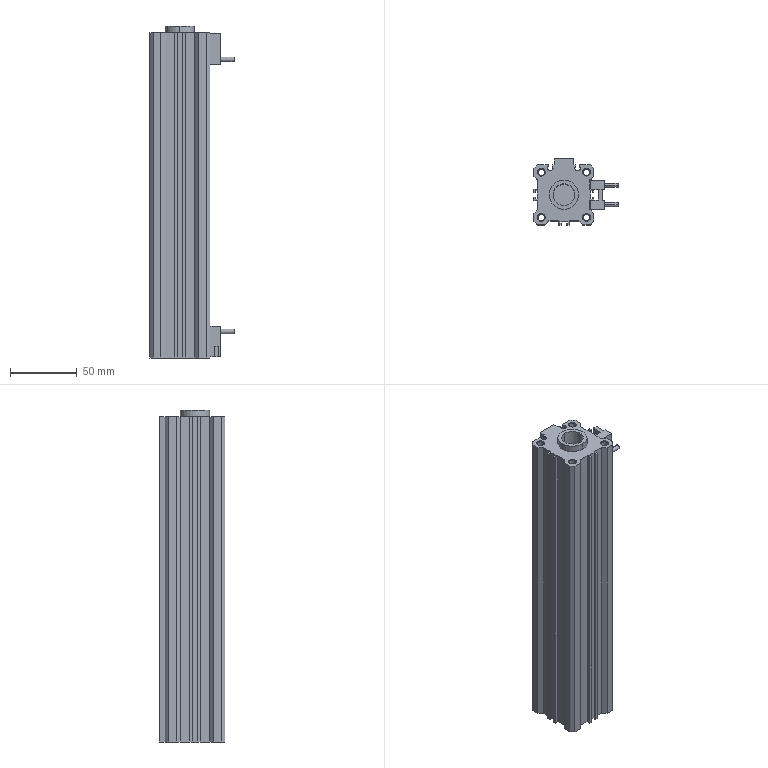Part | STEP file | A_CDQ2A32-200DC-F7NV(0)_Default | 1 solid | 140 faces | box 63.2 x 49.5 x 249.5 mm | volume 394520 mm3 | plane 88 | cylinder 30 | cone 20 | spline 2 | commonest cylinder face diameters 4.92 x8 4.2 x6 3.4 x4 8.57 x4 60 x4 16.4 x2